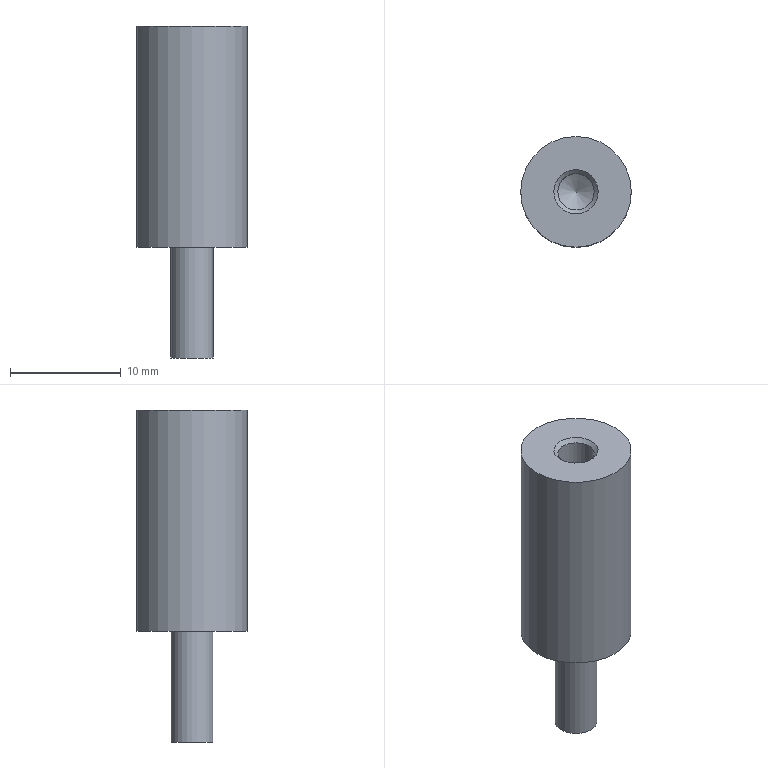Part | NX | features DATUM_CSYS 3, EXTRUDE 2, SKETCH 2, HOLE PACKAGE 1, SIMPLE HOLE 1, SYMBOLIC_THREAD 1 | 1 solid | 8 faces | box 10 x 10 x 30 mm | volume 1552 mm3 | cylinder 3 | plane 3 | cone 2 | commonest cylinder face diameters 3.3 x1 3.8 x1 10 x1
STEP:
#1=CARTESIAN_POINT('',(1.9,0.,10.));
#2=VERTEX_POINT('',#1);
#3=CARTESIAN_POINT('',(0.,0.,10.));
#4=DIRECTION('',(0.,0.,1.));
#5=DIRECTION('',(1.,0.,0.));
#6=AXIS2_PLACEMENT_3D('',#3,#4,#5);
#7=CIRCLE('',#6,1.9);
#8=EDGE_CURVE('',#2,#2,#7,.T.);
#9=ORIENTED_EDGE('',*,*,#8,.F.);
#10=EDGE_LOOP('',(#9));
#11=FACE_BOUND('',#10,.T.);
#12=CARTESIAN_POINT('',(1.9,0.,0.));
#13=VERTEX_POINT('',#12);
#14=CARTESIAN_POINT('',(0.,0.,0.));
#15=DIRECTION('',(0.,0.,1.));
#16=DIRECTION('',(1.,0.,0.));
#17=AXIS2_PLACEMENT_3D('',#14,#15,#16);
#18=CIRCLE('',#17,1.9);
#19=EDGE_CURVE('',#13,#13,#18,.T.);
#20=ORIENTED_EDGE('',*,*,#19,.T.);
#21=EDGE_LOOP('',(#20));
#22=FACE_BOUND('',#21,.T.);
#23=CARTESIAN_POINT('',(0.,0.,10.));
#24=DIRECTION('',(0.,0.,-1.));
#25=DIRECTION('',(-1.,0.,0.));
#26=AXIS2_PLACEMENT_3D('',#23,#24,#25);
#27=CYLINDRICAL_SURFACE('',#26,1.9);
#28=ADVANCED_FACE('',(#11,#22),#27,.T.);
#29=ORIENTED_EDGE('',*,*,#19,.F.);
#30=EDGE_LOOP('',(#29));
#31=FACE_BOUND('',#30,.T.);
#32=CARTESIAN_POINT('',(0.,0.,0.));
#33=DIRECTION('',(0.,0.,1.));
#34=DIRECTION('',(1.,0.,0.));
#35=AXIS2_PLACEMENT_3D('',#32,#33,#34);
#36=PLANE('',#35);
#37=ADVANCED_FACE('',(#31),#36,.F.);
#38=CARTESIAN_POINT('',(5.,0.,30.));
#39=VERTEX_POINT('',#38);
#40=CARTESIAN_POINT('',(0.,0.,30.));
#41=DIRECTION('',(0.,0.,1.));
#42=DIRECTION('',(1.,0.,0.));
#43=AXIS2_PLACEMENT_3D('',#40,#41,#42);
#44=CIRCLE('',#43,5.);
#45=EDGE_CURVE('',#39,#39,#44,.T.);
#46=ORIENTED_EDGE('',*,*,#45,.F.);
#47=EDGE_LOOP('',(#46));
#48=FACE_BOUND('',#47,.T.);
#49=CARTESIAN_POINT('',(5.,0.,10.));
#50=VERTEX_POINT('',#49);
#51=CARTESIAN_POINT('',(0.,0.,10.));
#52=DIRECTION('',(0.,0.,1.));
#53=DIRECTION('',(1.,0.,0.));
#54=AXIS2_PLACEMENT_3D('',#51,#52,#53);
#55=CIRCLE('',#54,5.);
#56=EDGE_CURVE('',#50,#50,#55,.T.);
#57=ORIENTED_EDGE('',*,*,#56,.T.);
#58=EDGE_LOOP('',(#57));
#59=FACE_BOUND('',#58,.T.);
#60=CARTESIAN_POINT('',(0.,0.,30.));
#61=DIRECTION('',(0.,0.,-1.));
#62=DIRECTION('',(-1.,0.,0.));
#63=AXIS2_PLACEMENT_3D('',#60,#61,#62);
#64=CYLINDRICAL_SURFACE('',#63,5.);
#65=ADVANCED_FACE('',(#48,#59),#64,.T.);
#66=CARTESIAN_POINT('',(2.,0.,30.));
#67=VERTEX_POINT('',#66);
#68=CARTESIAN_POINT('',(0.,0.,30.));
#69=DIRECTION('',(0.,0.,1.));
#70=DIRECTION('',(1.,0.,0.));
#71=AXIS2_PLACEMENT_3D('',#68,#69,#70);
#72=CIRCLE('',#71,2.);
#73=EDGE_CURVE('',#67,#67,#72,.F.);
#74=ORIENTED_EDGE('',*,*,#73,.T.);
#75=EDGE_LOOP('',(#74));
#76=FACE_BOUND('',#75,.T.);
#77=ORIENTED_EDGE('',*,*,#45,.T.);
#78=EDGE_LOOP('',(#77));
#79=FACE_BOUND('',#78,.T.);
#80=CARTESIAN_POINT('',(0.,0.,30.));
#81=DIRECTION('',(0.,0.,1.));
#82=DIRECTION('',(1.,0.,0.));
#83=AXIS2_PLACEMENT_3D('',#80,#81,#82);
#84=PLANE('',#83);
#85=ADVANCED_FACE('',(#76,#79),#84,.T.);
#86=ORIENTED_EDGE('',*,*,#8,.T.);
#87=EDGE_LOOP('',(#86));
#88=FACE_BOUND('',#87,.T.);
#89=ORIENTED_EDGE('',*,*,#56,.F.);
#90=EDGE_LOOP('',(#89));
#91=FACE_BOUND('',#90,.T.);
#92=CARTESIAN_POINT('',(0.,0.,10.));
#93=DIRECTION('',(0.,0.,1.));
#94=DIRECTION('',(1.,0.,0.));
#95=AXIS2_PLACEMENT_3D('',#92,#93,#94);
#96=PLANE('',#95);
#97=ADVANCED_FACE('',(#88,#91),#96,.F.);
#98=CARTESIAN_POINT('',(-1.65,0.,15.));
#99=VERTEX_POINT('',#98);
#100=CARTESIAN_POINT('',(0.,0.,15.));
#101=DIRECTION('',(0.,0.,-1.));
#102=DIRECTION('',(-1.,0.,0.));
#103=AXIS2_PLACEMENT_3D('',#100,#101,#102);
#104=CIRCLE('',#103,1.65);
#105=EDGE_CURVE('',#99,#99,#104,.F.);
#106=ORIENTED_EDGE('',*,*,#105,.T.);
#107=EDGE_LOOP('',(#106));
#108=FACE_BOUND('',#107,.T.);
#109=CARTESIAN_POINT('',(0.,0.,14.009));
#110=VERTEX_POINT('',#109);
#111=VERTEX_LOOP('',#110);
#112=FACE_BOUND('',#111,.T.);
#113=CARTESIAN_POINT('',(0.,0.,15.));
#114=DIRECTION('',(0.,0.,1.));
#115=DIRECTION('',(1.,0.,0.));
#116=AXIS2_PLACEMENT_3D('',#113,#114,#115);
#117=CONICAL_SURFACE('',#116,1.65,1.03);
#118=ADVANCED_FACE('',(#108,#112),#117,.F.);
#119=CARTESIAN_POINT('',(1.65,0.,29.65));
#120=VERTEX_POINT('',#119);
#121=CARTESIAN_POINT('',(0.,0.,29.65));
#122=DIRECTION('',(0.,0.,1.));
#123=DIRECTION('',(1.,0.,0.));
#124=AXIS2_PLACEMENT_3D('',#121,#122,#123);
#125=CIRCLE('',#124,1.65);
#126=EDGE_CURVE('',#120,#120,#125,.T.);
#127=ORIENTED_EDGE('',*,*,#126,.T.);
#128=EDGE_LOOP('',(#127));
#129=FACE_BOUND('',#128,.T.);
#130=ORIENTED_EDGE('',*,*,#105,.F.);
#131=EDGE_LOOP('',(#130));
#132=FACE_BOUND('',#131,.T.);
#133=CARTESIAN_POINT('',(0.,0.,30.));
#134=DIRECTION('',(0.,0.,-1.));
#135=DIRECTION('',(-1.,0.,0.));
#136=AXIS2_PLACEMENT_3D('',#133,#134,#135);
#137=CYLINDRICAL_SURFACE('',#136,1.65);
#138=ADVANCED_FACE('',(#129,#132),#137,.F.);
#139=ORIENTED_EDGE('',*,*,#126,.F.);
#140=EDGE_LOOP('',(#139));
#141=FACE_BOUND('',#140,.T.);
#142=ORIENTED_EDGE('',*,*,#73,.F.);
#143=EDGE_LOOP('',(#142));
#144=FACE_BOUND('',#143,.T.);
#145=CARTESIAN_POINT('',(0.,0.,30.));
#146=DIRECTION('',(0.,0.,1.));
#147=DIRECTION('',(1.,0.,0.));
#148=AXIS2_PLACEMENT_3D('',#145,#146,#147);
#149=CONICAL_SURFACE('',#148,2.,0.7854);
#150=ADVANCED_FACE('',(#141,#144),#149,.F.);
#151=CLOSED_SHELL('',(#28,#37,#65,#85,#97,#118,#138,#150));
#152=MANIFOLD_SOLID_BREP('',#151);
#153=(LENGTH_UNIT()NAMED_UNIT(*)SI_UNIT(.MILLI.,.METRE.));
#154=UNCERTAINTY_MEASURE_WITH_UNIT(LENGTH_MEASURE(0.00001),#153,'','');
#155=(NAMED_UNIT(*)PLANE_ANGLE_UNIT()SI_UNIT($,.RADIAN.));
#156=(NAMED_UNIT(*)SI_UNIT($,.STERADIAN.)SOLID_ANGLE_UNIT());
#157=(GEOMETRIC_REPRESENTATION_CONTEXT(3)GLOBAL_UNCERTAINTY_ASSIGNED_CONTEXT((#154))GLOBAL_UNIT_ASSIGNED_CONTEXT((#153,#155,#156))REPRESENTATION_CONTEXT('',''));
#158=ADVANCED_BREP_SHAPE_REPRESENTATION('',(#152),#157);